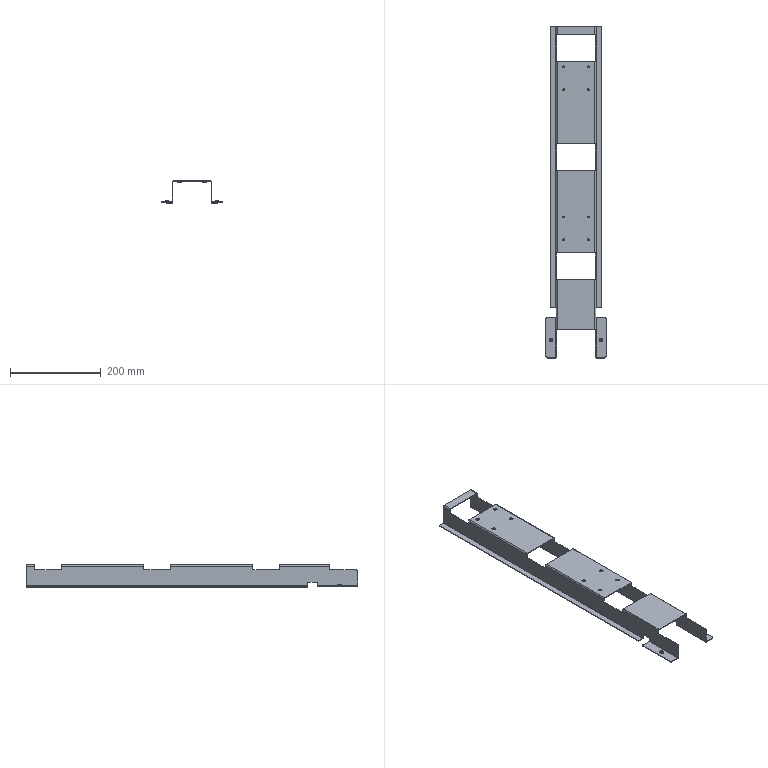Part | SolidWorks | features ICE 5, EdgeFlange 3, LPattern 3, 3DProfileFeature 2, Fillet 2, HoleWzd 2, SMBaseFlange 2, FlatPattern 1, MirrorPattern 1, SheetMetal 1 | 1 solid | 176 faces | box 132 x 730 x 48.5 mm | volume 188452 mm3 | plane 106 | cylinder 70 | commonest cylinder face diameters 4.2 x16 8.64 x16 1.6 x12 4.6 x12 8 x6 3.3 x4